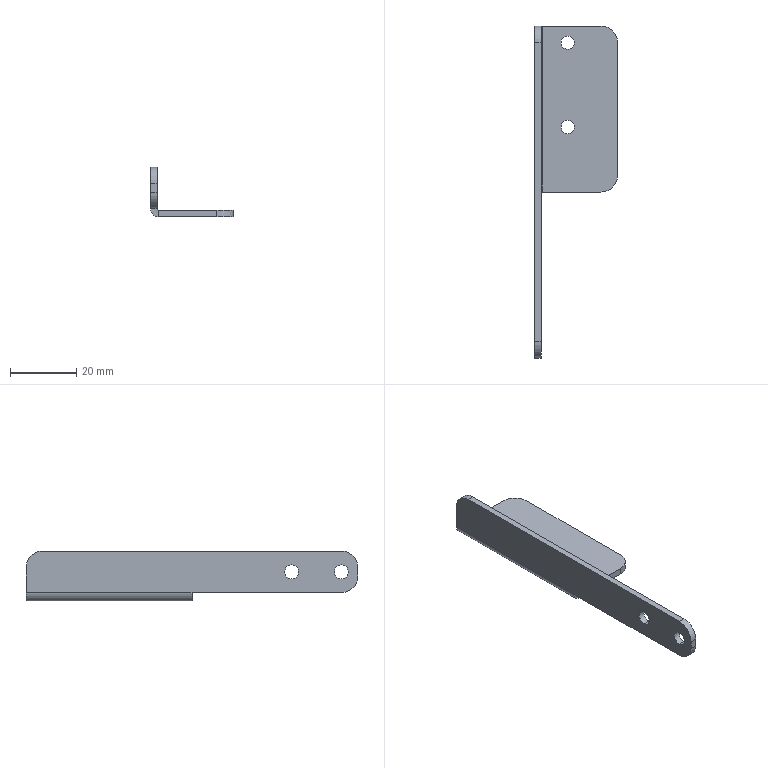Part | SolidWorks | features HoleWzd 2, DeleteBody 1, EdgeFlange 1, Fillet 1, FlatPattern 1, MirrorSolid 1, SMBaseFlange 1, SheetMetal 1 | 1 solid | 28 faces | box 25 x 100 x 15 mm | volume 4826 mm3 | cylinder 15 | plane 13 | commonest cylinder face diameters 10 x5 4 x4 4.2 x4 1 x1 5 x1
STEP:
#1=CARTESIAN_POINT('',(0.,-30.,8.85));
#2=VERTEX_POINT('',#1);
#3=CARTESIAN_POINT('',(0.,-30.,4.65));
#4=VERTEX_POINT('',#3);
#5=CARTESIAN_POINT('',(0.,-30.,6.75));
#6=DIRECTION('',(1.,0.,0.));
#7=DIRECTION('',(0.,0.,-1.));
#8=AXIS2_PLACEMENT_3D('',#5,#6,#7);
#9=CIRCLE('',#8,2.1);
#10=EDGE_CURVE('',#2,#4,#9,.T.);
#11=ORIENTED_EDGE('',*,*,#10,.F.);
#12=CARTESIAN_POINT('',(2.,-30.,8.85));
#13=VERTEX_POINT('',#12);
#14=CARTESIAN_POINT('',(2.,-30.,8.85));
#15=DIRECTION('',(1.,0.,0.));
#16=VECTOR('',#15,1000.);
#17=LINE('',#14,#16);
#18=EDGE_CURVE('',#2,#13,#17,.T.);
#19=ORIENTED_EDGE('',*,*,#18,.T.);
#20=CARTESIAN_POINT('',(2.,-30.,4.65));
#21=VERTEX_POINT('',#20);
#22=CARTESIAN_POINT('',(2.,-30.,6.75));
#23=DIRECTION('',(1.,0.,0.));
#24=DIRECTION('',(0.,0.,-1.));
#25=AXIS2_PLACEMENT_3D('',#22,#23,#24);
#26=CIRCLE('',#25,2.1);
#27=EDGE_CURVE('',#13,#21,#26,.T.);
#28=ORIENTED_EDGE('',*,*,#27,.T.);
#29=CARTESIAN_POINT('',(2.,-30.,4.65));
#30=DIRECTION('',(1.,0.,0.));
#31=VECTOR('',#30,1000.);
#32=LINE('',#29,#31);
#33=EDGE_CURVE('',#4,#21,#32,.T.);
#34=ORIENTED_EDGE('',*,*,#33,.F.);
#35=EDGE_LOOP('',(#11,#19,#28,#34));
#36=FACE_OUTER_BOUND('',#35,.T.);
#37=CARTESIAN_POINT('',(2.,-30.,6.75));
#38=DIRECTION('',(1.,0.,0.));
#39=DIRECTION('',(0.,0.,-1.));
#40=AXIS2_PLACEMENT_3D('',#37,#38,#39);
#41=CYLINDRICAL_SURFACE('',#40,2.1);
#42=ADVANCED_FACE('',(#36),#41,.F.);
#43=CARTESIAN_POINT('',(0.,-45.,8.85));
#44=VERTEX_POINT('',#43);
#45=CARTESIAN_POINT('',(0.,-45.,4.65));
#46=VERTEX_POINT('',#45);
#47=CARTESIAN_POINT('',(0.,-45.,6.75));
#48=DIRECTION('',(1.,0.,0.));
#49=DIRECTION('',(0.,0.,-1.));
#50=AXIS2_PLACEMENT_3D('',#47,#48,#49);
#51=CIRCLE('',#50,2.1);
#52=EDGE_CURVE('',#44,#46,#51,.T.);
#53=ORIENTED_EDGE('',*,*,#52,.F.);
#54=CARTESIAN_POINT('',(2.,-45.,8.85));
#55=VERTEX_POINT('',#54);
#56=CARTESIAN_POINT('',(2.,-45.,8.85));
#57=DIRECTION('',(1.,0.,0.));
#58=VECTOR('',#57,1000.);
#59=LINE('',#56,#58);
#60=EDGE_CURVE('',#44,#55,#59,.T.);
#61=ORIENTED_EDGE('',*,*,#60,.T.);
#62=CARTESIAN_POINT('',(2.,-45.,4.65));
#63=VERTEX_POINT('',#62);
#64=CARTESIAN_POINT('',(2.,-45.,6.75));
#65=DIRECTION('',(1.,0.,0.));
#66=DIRECTION('',(0.,0.,-1.));
#67=AXIS2_PLACEMENT_3D('',#64,#65,#66);
#68=CIRCLE('',#67,2.1);
#69=EDGE_CURVE('',#55,#63,#68,.T.);
#70=ORIENTED_EDGE('',*,*,#69,.T.);
#71=CARTESIAN_POINT('',(2.,-45.,4.65));
#72=DIRECTION('',(1.,0.,0.));
#73=VECTOR('',#72,1000.);
#74=LINE('',#71,#73);
#75=EDGE_CURVE('',#46,#63,#74,.T.);
#76=ORIENTED_EDGE('',*,*,#75,.F.);
#77=EDGE_LOOP('',(#53,#61,#70,#76));
#78=FACE_OUTER_BOUND('',#77,.T.);
#79=CARTESIAN_POINT('',(2.,-45.,6.75));
#80=DIRECTION('',(1.,0.,0.));
#81=DIRECTION('',(0.,0.,-1.));
#82=AXIS2_PLACEMENT_3D('',#79,#80,#81);
#83=CYLINDRICAL_SURFACE('',#82,2.1);
#84=ADVANCED_FACE('',(#78),#83,.F.);
#85=CARTESIAN_POINT('',(8.,45.,-2.));
#86=VERTEX_POINT('',#85);
#87=CARTESIAN_POINT('',(12.,45.,-2.));
#88=VERTEX_POINT('',#87);
#89=CARTESIAN_POINT('',(10.,45.,-2.));
#90=DIRECTION('',(0.,0.,1.));
#91=DIRECTION('',(1.,0.,0.));
#92=AXIS2_PLACEMENT_3D('',#89,#90,#91);
#93=CIRCLE('',#92,2.);
#94=EDGE_CURVE('',#86,#88,#93,.T.);
#95=ORIENTED_EDGE('',*,*,#94,.F.);
#96=CARTESIAN_POINT('',(8.,45.,0.));
#97=VERTEX_POINT('',#96);
#98=CARTESIAN_POINT('',(8.,45.,0.));
#99=DIRECTION('',(0.,0.,1.));
#100=VECTOR('',#99,1000.);
#101=LINE('',#98,#100);
#102=EDGE_CURVE('',#86,#97,#101,.T.);
#103=ORIENTED_EDGE('',*,*,#102,.T.);
#104=CARTESIAN_POINT('',(12.,45.,0.));
#105=VERTEX_POINT('',#104);
#106=CARTESIAN_POINT('',(10.,45.,0.));
#107=DIRECTION('',(0.,0.,1.));
#108=DIRECTION('',(1.,0.,0.));
#109=AXIS2_PLACEMENT_3D('',#106,#107,#108);
#110=CIRCLE('',#109,2.);
#111=EDGE_CURVE('',#97,#105,#110,.T.);
#112=ORIENTED_EDGE('',*,*,#111,.T.);
#113=CARTESIAN_POINT('',(12.,45.,0.));
#114=DIRECTION('',(0.,0.,1.));
#115=VECTOR('',#114,1000.);
#116=LINE('',#113,#115);
#117=EDGE_CURVE('',#88,#105,#116,.T.);
#118=ORIENTED_EDGE('',*,*,#117,.F.);
#119=EDGE_LOOP('',(#95,#103,#112,#118));
#120=FACE_OUTER_BOUND('',#119,.T.);
#121=CARTESIAN_POINT('',(10.,45.,0.));
#122=DIRECTION('',(0.,0.,1.));
#123=DIRECTION('',(1.,0.,0.));
#124=AXIS2_PLACEMENT_3D('',#121,#122,#123);
#125=CYLINDRICAL_SURFACE('',#124,2.);
#126=ADVANCED_FACE('',(#120),#125,.F.);
#127=CARTESIAN_POINT('',(8.,19.6,-2.));
#128=VERTEX_POINT('',#127);
#129=CARTESIAN_POINT('',(12.,19.6,-2.));
#130=VERTEX_POINT('',#129);
#131=CARTESIAN_POINT('',(10.,19.6,-2.));
#132=DIRECTION('',(0.,0.,1.));
#133=DIRECTION('',(1.,0.,0.));
#134=AXIS2_PLACEMENT_3D('',#131,#132,#133);
#135=CIRCLE('',#134,2.);
#136=EDGE_CURVE('',#128,#130,#135,.T.);
#137=ORIENTED_EDGE('',*,*,#136,.F.);
#138=CARTESIAN_POINT('',(8.,19.6,0.));
#139=VERTEX_POINT('',#138);
#140=CARTESIAN_POINT('',(8.,19.6,0.));
#141=DIRECTION('',(0.,0.,1.));
#142=VECTOR('',#141,1000.);
#143=LINE('',#140,#142);
#144=EDGE_CURVE('',#128,#139,#143,.T.);
#145=ORIENTED_EDGE('',*,*,#144,.T.);
#146=CARTESIAN_POINT('',(12.,19.6,0.));
#147=VERTEX_POINT('',#146);
#148=CARTESIAN_POINT('',(10.,19.6,0.));
#149=DIRECTION('',(0.,0.,1.));
#150=DIRECTION('',(1.,0.,0.));
#151=AXIS2_PLACEMENT_3D('',#148,#149,#150);
#152=CIRCLE('',#151,2.);
#153=EDGE_CURVE('',#139,#147,#152,.T.);
#154=ORIENTED_EDGE('',*,*,#153,.T.);
#155=CARTESIAN_POINT('',(12.,19.6,0.));
#156=DIRECTION('',(0.,0.,1.));
#157=VECTOR('',#156,1000.);
#158=LINE('',#155,#157);
#159=EDGE_CURVE('',#130,#147,#158,.T.);
#160=ORIENTED_EDGE('',*,*,#159,.F.);
#161=EDGE_LOOP('',(#137,#145,#154,#160));
#162=FACE_OUTER_BOUND('',#161,.T.);
#163=CARTESIAN_POINT('',(10.,19.6,0.));
#164=DIRECTION('',(0.,0.,1.));
#165=DIRECTION('',(1.,0.,0.));
#166=AXIS2_PLACEMENT_3D('',#163,#164,#165);
#167=CYLINDRICAL_SURFACE('',#166,2.);
#168=ADVANCED_FACE('',(#162),#167,.F.);
#169=CARTESIAN_POINT('',(2.5,0.,-2.));
#170=VERTEX_POINT('',#169);
#171=CARTESIAN_POINT('',(20.,0.,-2.));
#172=VERTEX_POINT('',#171);
#173=CARTESIAN_POINT('',(0.,0.,-2.));
#174=DIRECTION('',(1.,0.,0.));
#175=VECTOR('',#174,1000.);
#176=LINE('',#173,#175);
#177=EDGE_CURVE('',#170,#172,#176,.T.);
#178=ORIENTED_EDGE('',*,*,#177,.T.);
#179=CARTESIAN_POINT('',(20.,0.,0.));
#180=VERTEX_POINT('',#179);
#181=CARTESIAN_POINT('',(20.,0.,-2.));
#182=DIRECTION('',(0.,0.,1.));
#183=VECTOR('',#182,1000.);
#184=LINE('',#181,#183);
#185=EDGE_CURVE('',#172,#180,#184,.T.);
#186=ORIENTED_EDGE('',*,*,#185,.T.);
#187=CARTESIAN_POINT('',(2.5,0.,0.));
#188=VERTEX_POINT('',#187);
#189=CARTESIAN_POINT('',(0.,0.,0.));
#190=DIRECTION('',(1.,0.,0.));
#191=VECTOR('',#190,1000.);
#192=LINE('',#189,#191);
#193=EDGE_CURVE('',#188,#180,#192,.T.);
#194=ORIENTED_EDGE('',*,*,#193,.F.);
#195=CARTESIAN_POINT('',(2.5,0.,0.));
#196=DIRECTION('',(0.,0.,-1.));
#197=VECTOR('',#196,1000.);
#198=LINE('',#195,#197);
#199=EDGE_CURVE('',#188,#170,#198,.T.);
#200=ORIENTED_EDGE('',*,*,#199,.T.);
#201=EDGE_LOOP('',(#178,#186,#194,#200));
#202=FACE_OUTER_BOUND('',#201,.T.);
#203=CARTESIAN_POINT('',(0.,0.,-2.));
#204=DIRECTION('',(0.,-1.,0.));
#205=DIRECTION('',(0.,0.,-1.));
#206=AXIS2_PLACEMENT_3D('',#203,#204,#205);
#207=PLANE('',#206);
#208=ADVANCED_FACE('',(#202),#207,.T.);
#209=CARTESIAN_POINT('',(10.,45.,-2.));
#210=DIRECTION('',(0.,0.,1.));
#211=DIRECTION('',(1.,0.,0.));
#212=AXIS2_PLACEMENT_3D('',#209,#210,#211);
#213=CIRCLE('',#212,2.);
#214=EDGE_CURVE('',#88,#86,#213,.T.);
#215=ORIENTED_EDGE('',*,*,#214,.T.);
#216=ORIENTED_EDGE('',*,*,#94,.T.);
#217=EDGE_LOOP('',(#215,#216));
#218=FACE_BOUND('',#217,.T.);
#219=CARTESIAN_POINT('',(10.,19.6,-2.));
#220=DIRECTION('',(0.,0.,1.));
#221=DIRECTION('',(1.,0.,0.));
#222=AXIS2_PLACEMENT_3D('',#219,#220,#221);
#223=CIRCLE('',#222,2.);
#224=EDGE_CURVE('',#130,#128,#223,.T.);
#225=ORIENTED_EDGE('',*,*,#224,.T.);
#226=ORIENTED_EDGE('',*,*,#136,.T.);
#227=EDGE_LOOP('',(#225,#226));
#228=FACE_BOUND('',#227,.T.);
#229=CARTESIAN_POINT('',(25.,5.,-2.));
#230=VERTEX_POINT('',#229);
#231=CARTESIAN_POINT('',(25.,45.,-2.));
#232=VERTEX_POINT('',#231);
#233=CARTESIAN_POINT('',(25.,50.,-2.));
#234=DIRECTION('',(0.,1.,0.));
#235=VECTOR('',#234,1000.);
#236=LINE('',#233,#235);
#237=EDGE_CURVE('',#230,#232,#236,.T.);
#238=ORIENTED_EDGE('',*,*,#237,.F.);
#239=CARTESIAN_POINT('',(20.,5.,-2.));
#240=DIRECTION('',(0.,0.,-1.));
#241=DIRECTION('',(-1.,0.,0.));
#242=AXIS2_PLACEMENT_3D('',#239,#240,#241);
#243=CIRCLE('',#242,5.);
#244=EDGE_CURVE('',#230,#172,#243,.T.);
#245=ORIENTED_EDGE('',*,*,#244,.T.);
#246=ORIENTED_EDGE('',*,*,#177,.F.);
#247=CARTESIAN_POINT('',(2.5,50.,-2.));
#248=VERTEX_POINT('',#247);
#249=CARTESIAN_POINT('',(2.5,0.,-2.));
#250=DIRECTION('',(0.,1.,0.));
#251=VECTOR('',#250,1000.);
#252=LINE('',#249,#251);
#253=EDGE_CURVE('',#170,#248,#252,.T.);
#254=ORIENTED_EDGE('',*,*,#253,.T.);
#255=CARTESIAN_POINT('',(20.,50.,-2.));
#256=VERTEX_POINT('',#255);
#257=CARTESIAN_POINT('',(0.,50.,-2.));
#258=DIRECTION('',(-1.,0.,0.));
#259=VECTOR('',#258,1000.);
#260=LINE('',#257,#259);
#261=EDGE_CURVE('',#256,#248,#260,.T.);
#262=ORIENTED_EDGE('',*,*,#261,.F.);
#263=CARTESIAN_POINT('',(20.,45.,-2.));
#264=DIRECTION('',(0.,0.,-1.));
#265=DIRECTION('',(-1.,0.,0.));
#266=AXIS2_PLACEMENT_3D('',#263,#264,#265);
#267=CIRCLE('',#266,5.);
#268=EDGE_CURVE('',#256,#232,#267,.T.);
#269=ORIENTED_EDGE('',*,*,#268,.T.);
#270=EDGE_LOOP('',(#238,#245,#246,#254,#262,#269));
#271=FACE_OUTER_BOUND('',#270,.T.);
#272=CARTESIAN_POINT('',(0.,0.,-2.));
#273=DIRECTION('',(0.,0.,-1.));
#274=DIRECTION('',(-1.,0.,0.));
#275=AXIS2_PLACEMENT_3D('',#272,#273,#274);
#276=PLANE('',#275);
#277=ADVANCED_FACE('',(#218,#228,#271),#276,.T.);
#278=CARTESIAN_POINT('',(10.,19.6,0.));
#279=DIRECTION('',(0.,0.,1.));
#280=DIRECTION('',(1.,0.,0.));
#281=AXIS2_PLACEMENT_3D('',#278,#279,#280);
#282=CIRCLE('',#281,2.);
#283=EDGE_CURVE('',#147,#139,#282,.T.);
#284=ORIENTED_EDGE('',*,*,#283,.F.);
#285=ORIENTED_EDGE('',*,*,#153,.F.);
#286=EDGE_LOOP('',(#284,#285));
#287=FACE_BOUND('',#286,.T.);
#288=CARTESIAN_POINT('',(10.,45.,0.));
#289=DIRECTION('',(0.,0.,1.));
#290=DIRECTION('',(1.,0.,0.));
#291=AXIS2_PLACEMENT_3D('',#288,#289,#290);
#292=CIRCLE('',#291,2.);
#293=EDGE_CURVE('',#105,#97,#292,.T.);
#294=ORIENTED_EDGE('',*,*,#293,.F.);
#295=ORIENTED_EDGE('',*,*,#111,.F.);
#296=EDGE_LOOP('',(#294,#295));
#297=FACE_BOUND('',#296,.T.);
#298=ORIENTED_EDGE('',*,*,#193,.T.);
#299=CARTESIAN_POINT('',(25.,5.,0.));
#300=VERTEX_POINT('',#299);
#301=CARTESIAN_POINT('',(20.,5.,0.));
#302=DIRECTION('',(0.,0.,1.));
#303=DIRECTION('',(-1.,0.,0.));
#304=AXIS2_PLACEMENT_3D('',#301,#302,#303);
#305=CIRCLE('',#304,5.);
#306=EDGE_CURVE('',#180,#300,#305,.T.);
#307=ORIENTED_EDGE('',*,*,#306,.T.);
#308=CARTESIAN_POINT('',(25.,45.,0.));
#309=VERTEX_POINT('',#308);
#310=CARTESIAN_POINT('',(25.,50.,0.));
#311=DIRECTION('',(0.,1.,0.));
#312=VECTOR('',#311,1000.);
#313=LINE('',#310,#312);
#314=EDGE_CURVE('',#300,#309,#313,.T.);
#315=ORIENTED_EDGE('',*,*,#314,.T.);
#316=CARTESIAN_POINT('',(20.,50.,0.));
#317=VERTEX_POINT('',#316);
#318=CARTESIAN_POINT('',(20.,45.,0.));
#319=DIRECTION('',(0.,0.,1.));
#320=DIRECTION('',(-1.,0.,0.));
#321=AXIS2_PLACEMENT_3D('',#318,#319,#320);
#322=CIRCLE('',#321,5.);
#323=EDGE_CURVE('',#309,#317,#322,.T.);
#324=ORIENTED_EDGE('',*,*,#323,.T.);
#325=CARTESIAN_POINT('',(2.5,50.,0.));
#326=VERTEX_POINT('',#325);
#327=CARTESIAN_POINT('',(0.,50.,0.));
#328=DIRECTION('',(-1.,0.,0.));
#329=VECTOR('',#328,1000.);
#330=LINE('',#327,#329);
#331=EDGE_CURVE('',#317,#326,#330,.T.);
#332=ORIENTED_EDGE('',*,*,#331,.T.);
#333=CARTESIAN_POINT('',(2.5,0.,0.));
#334=DIRECTION('',(0.,1.,0.));
#335=VECTOR('',#334,1000.);
#336=LINE('',#333,#335);
#337=EDGE_CURVE('',#188,#326,#336,.T.);
#338=ORIENTED_EDGE('',*,*,#337,.F.);
#339=EDGE_LOOP('',(#298,#307,#315,#324,#332,#338));
#340=FACE_OUTER_BOUND('',#339,.T.);
#341=CARTESIAN_POINT('',(0.,0.,0.));
#342=DIRECTION('',(0.,0.,-1.));
#343=DIRECTION('',(-1.,0.,0.));
#344=AXIS2_PLACEMENT_3D('',#341,#342,#343);
#345=PLANE('',#344);
#346=ADVANCED_FACE('',(#287,#297,#340),#345,.F.);
#347=ORIENTED_EDGE('',*,*,#331,.F.);
#348=CARTESIAN_POINT('',(20.,50.,-2.));
#349=DIRECTION('',(0.,0.,-1.));
#350=VECTOR('',#349,1000.);
#351=LINE('',#348,#350);
#352=EDGE_CURVE('',#317,#256,#351,.T.);
#353=ORIENTED_EDGE('',*,*,#352,.T.);
#354=ORIENTED_EDGE('',*,*,#261,.T.);
#355=CARTESIAN_POINT('',(2.5,50.,0.));
#356=DIRECTION('',(0.,0.,-1.));
#357=VECTOR('',#356,1000.);
#358=LINE('',#355,#357);
#359=EDGE_CURVE('',#326,#248,#358,.T.);
#360=ORIENTED_EDGE('',*,*,#359,.F.);
#361=EDGE_LOOP('',(#347,#353,#354,#360));
#362=FACE_OUTER_BOUND('',#361,.T.);
#363=CARTESIAN_POINT('',(0.,50.,-2.));
#364=DIRECTION('',(0.,1.,0.));
#365=DIRECTION('',(0.,0.,1.));
#366=AXIS2_PLACEMENT_3D('',#363,#364,#365);
#367=PLANE('',#366);
#368=ADVANCED_FACE('',(#362),#367,.T.);
#369=ORIENTED_EDGE('',*,*,#314,.F.);
#370=CARTESIAN_POINT('',(25.,5.,-2.));
#371=DIRECTION('',(0.,0.,-1.));
#372=VECTOR('',#371,1000.);
#373=LINE('',#370,#372);
#374=EDGE_CURVE('',#300,#230,#373,.T.);
#375=ORIENTED_EDGE('',*,*,#374,.T.);
#376=ORIENTED_EDGE('',*,*,#237,.T.);
#377=CARTESIAN_POINT('',(25.,45.,-2.));
#378=DIRECTION('',(0.,0.,1.));
#379=VECTOR('',#378,1000.);
#380=LINE('',#377,#379);
#381=EDGE_CURVE('',#232,#309,#380,.T.);
#382=ORIENTED_EDGE('',*,*,#381,.T.);
#383=EDGE_LOOP('',(#369,#375,#376,#382));
#384=FACE_OUTER_BOUND('',#383,.T.);
#385=CARTESIAN_POINT('',(25.,50.,-2.));
#386=DIRECTION('',(1.,0.,0.));
#387=DIRECTION('',(0.,1.,0.));
#388=AXIS2_PLACEMENT_3D('',#385,#386,#387);
#389=PLANE('',#388);
#390=ADVANCED_FACE('',(#384),#389,.T.);
#391=ORIENTED_EDGE('',*,*,#144,.F.);
#392=ORIENTED_EDGE('',*,*,#224,.F.);
#393=ORIENTED_EDGE('',*,*,#159,.T.);
#394=ORIENTED_EDGE('',*,*,#283,.T.);
#395=EDGE_LOOP('',(#391,#392,#393,#394));
#396=FACE_OUTER_BOUND('',#395,.T.);
#397=CARTESIAN_POINT('',(10.,19.6,0.));
#398=DIRECTION('',(0.,0.,1.));
#399=DIRECTION('',(1.,0.,0.));
#400=AXIS2_PLACEMENT_3D('',#397,#398,#399);
#401=CYLINDRICAL_SURFACE('',#400,2.);
#402=ADVANCED_FACE('',(#396),#401,.F.);
#403=ORIENTED_EDGE('',*,*,#102,.F.);
#404=ORIENTED_EDGE('',*,*,#214,.F.);
#405=ORIENTED_EDGE('',*,*,#117,.T.);
#406=ORIENTED_EDGE('',*,*,#293,.T.);
#407=EDGE_LOOP('',(#403,#404,#405,#406));
#408=FACE_OUTER_BOUND('',#407,.T.);
#409=CARTESIAN_POINT('',(10.,45.,0.));
#410=DIRECTION('',(0.,0.,1.));
#411=DIRECTION('',(1.,0.,0.));
#412=AXIS2_PLACEMENT_3D('',#409,#410,#411);
#413=CYLINDRICAL_SURFACE('',#412,2.);
#414=ADVANCED_FACE('',(#408),#413,.F.);
#415=CARTESIAN_POINT('',(2.,50.,0.5));
#416=VERTEX_POINT('',#415);
#417=CARTESIAN_POINT('',(0.,50.,0.5));
#418=VERTEX_POINT('',#417);
#419=CARTESIAN_POINT('',(0.,50.,0.5));
#420=DIRECTION('',(-1.,0.,0.));
#421=VECTOR('',#420,1000.);
#422=LINE('',#419,#421);
#423=EDGE_CURVE('',#416,#418,#422,.T.);
#424=ORIENTED_EDGE('',*,*,#423,.F.);
#425=CARTESIAN_POINT('',(2.5,50.,0.5));
#426=DIRECTION('',(0.,1.,0.));
#427=DIRECTION('',(0.,0.,-1.));
#428=AXIS2_PLACEMENT_3D('',#425,#426,#427);
#429=CIRCLE('',#428,0.5);
#430=EDGE_CURVE('',#326,#416,#429,.T.);
#431=ORIENTED_EDGE('',*,*,#430,.F.);
#432=ORIENTED_EDGE('',*,*,#359,.T.);
#433=CARTESIAN_POINT('',(2.5,50.,0.5));
#434=DIRECTION('',(0.,1.,0.));
#435=DIRECTION('',(0.,0.,-1.));
#436=AXIS2_PLACEMENT_3D('',#433,#434,#435);
#437=CIRCLE('',#436,2.5);
#438=EDGE_CURVE('',#248,#418,#437,.T.);
#439=ORIENTED_EDGE('',*,*,#438,.T.);
#440=EDGE_LOOP('',(#424,#431,#432,#439));
#441=FACE_OUTER_BOUND('',#440,.T.);
#442=CARTESIAN_POINT('',(2.5,50.,0.5));
#443=DIRECTION('',(0.,1.,0.));
#444=DIRECTION('',(0.,0.,1.));
#445=AXIS2_PLACEMENT_3D('',#442,#443,#444);
#446=PLANE('',#445);
#447=ADVANCED_FACE('',(#441),#446,.T.);
#448=CARTESIAN_POINT('',(2.,0.,0.5));
#449=VERTEX_POINT('',#448);
#450=CARTESIAN_POINT('',(2.5,0.,0.5));
#451=DIRECTION('',(0.,-1.,0.));
#452=DIRECTION('',(0.,0.,-1.));
#453=AXIS2_PLACEMENT_3D('',#450,#451,#452);
#454=CIRCLE('',#453,0.5);
#455=EDGE_CURVE('',#449,#188,#454,.T.);
#456=ORIENTED_EDGE('',*,*,#455,.F.);
#457=CARTESIAN_POINT('',(0.,0.,0.5));
#458=VERTEX_POINT('',#457);
#459=CARTESIAN_POINT('',(2.,0.,0.5));
#460=DIRECTION('',(-1.,0.,0.));
#461=VECTOR('',#460,1000.);
#462=LINE('',#459,#461);
#463=EDGE_CURVE('',#449,#458,#462,.T.);
#464=ORIENTED_EDGE('',*,*,#463,.T.);
#465=CARTESIAN_POINT('',(2.5,0.,0.5));
#466=DIRECTION('',(0.,-1.,0.));
#467=DIRECTION('',(0.,0.,-1.));
#468=AXIS2_PLACEMENT_3D('',#465,#466,#467);
#469=CIRCLE('',#468,2.5);
#470=EDGE_CURVE('',#458,#170,#469,.T.);
#471=ORIENTED_EDGE('',*,*,#470,.T.);
#472=ORIENTED_EDGE('',*,*,#199,.F.);
#473=EDGE_LOOP('',(#456,#464,#471,#472));
#474=FACE_OUTER_BOUND('',#473,.T.);
#475=CARTESIAN_POINT('',(2.5,0.,0.5));
#476=DIRECTION('',(0.,1.,0.));
#477=DIRECTION('',(0.,0.,1.));
#478=AXIS2_PLACEMENT_3D('',#475,#476,#477);
#479=PLANE('',#478);
#480=ADVANCED_FACE('',(#474),#479,.F.);
#481=ORIENTED_EDGE('',*,*,#253,.F.);
#482=ORIENTED_EDGE('',*,*,#470,.F.);
#483=CARTESIAN_POINT('',(0.,0.,0.5));
#484=DIRECTION('',(0.,-1.,0.));
#485=VECTOR('',#484,1000.);
#486=LINE('',#483,#485);
#487=EDGE_CURVE('',#418,#458,#486,.T.);
#488=ORIENTED_EDGE('',*,*,#487,.F.);
#489=ORIENTED_EDGE('',*,*,#438,.F.);
#490=EDGE_LOOP('',(#481,#482,#488,#489));
#491=FACE_OUTER_BOUND('',#490,.T.);
#492=CARTESIAN_POINT('',(2.5,0.,0.5));
#493=DIRECTION('',(0.,-1.,0.));
#494=DIRECTION('',(-1.,0.,0.));
#495=AXIS2_PLACEMENT_3D('',#492,#493,#494);
#496=CYLINDRICAL_SURFACE('',#495,2.5);
#497=ADVANCED_FACE('',(#491),#496,.T.);
#498=ORIENTED_EDGE('',*,*,#337,.T.);
#499=ORIENTED_EDGE('',*,*,#430,.T.);
#500=CARTESIAN_POINT('',(2.,50.,0.5));
#501=DIRECTION('',(0.,-1.,0.));
#502=VECTOR('',#501,1000.);
#503=LINE('',#500,#502);
#504=EDGE_CURVE('',#416,#449,#503,.T.);
#505=ORIENTED_EDGE('',*,*,#504,.T.);
#506=ORIENTED_EDGE('',*,*,#455,.T.);
#507=EDGE_LOOP('',(#498,#499,#505,#506));
#508=FACE_OUTER_BOUND('',#507,.T.);
#509=CARTESIAN_POINT('',(2.5,0.,0.5));
#510=DIRECTION('',(0.,-1.,0.));
#511=DIRECTION('',(-1.,0.,0.));
#512=AXIS2_PLACEMENT_3D('',#509,#510,#511);
#513=CYLINDRICAL_SURFACE('',#512,0.5);
#514=ADVANCED_FACE('',(#508),#513,.F.);
#515=CARTESIAN_POINT('',(2.,-45.,0.5));
#516=VERTEX_POINT('',#515);
#517=CARTESIAN_POINT('',(2.,50.,0.5));
#518=DIRECTION('',(0.,-1.,0.));
#519=VECTOR('',#518,1000.);
#520=LINE('',#517,#519);
#521=EDGE_CURVE('',#449,#516,#520,.T.);
#522=ORIENTED_EDGE('',*,*,#521,.T.);
#523=CARTESIAN_POINT('',(0.,-45.,0.5));
#524=VERTEX_POINT('',#523);
#525=CARTESIAN_POINT('',(0.,-45.,0.5));
#526=DIRECTION('',(-1.,0.,0.));
#527=VECTOR('',#526,1000.);
#528=LINE('',#525,#527);
#529=EDGE_CURVE('',#516,#524,#528,.T.);
#530=ORIENTED_EDGE('',*,*,#529,.T.);
#531=CARTESIAN_POINT('',(0.,50.,0.5));
#532=DIRECTION('',(0.,1.,0.));
#533=VECTOR('',#532,1000.);
#534=LINE('',#531,#533);
#535=EDGE_CURVE('',#524,#458,#534,.T.);
#536=ORIENTED_EDGE('',*,*,#535,.T.);
#537=ORIENTED_EDGE('',*,*,#463,.F.);
#538=EDGE_LOOP('',(#522,#530,#536,#537));
#539=FACE_OUTER_BOUND('',#538,.T.);
#540=CARTESIAN_POINT('',(2.,50.,0.5));
#541=DIRECTION('',(0.,0.,-1.));
#542=DIRECTION('',(-1.,0.,0.));
#543=AXIS2_PLACEMENT_3D('',#540,#541,#542);
#544=PLANE('',#543);
#545=ADVANCED_FACE('',(#539),#544,.T.);
#546=CARTESIAN_POINT('',(0.,50.,8.));
#547=VERTEX_POINT('',#546);
#548=CARTESIAN_POINT('',(0.,50.,0.));
#549=DIRECTION('',(0.,0.,-1.));
#550=VECTOR('',#549,1000.);
#551=LINE('',#548,#550);
#552=EDGE_CURVE('',#547,#418,#551,.T.);
#553=ORIENTED_EDGE('',*,*,#552,.F.);
#554=CARTESIAN_POINT('',(2.,50.,8.));
#555=VERTEX_POINT('',#554);
#556=CARTESIAN_POINT('',(0.,50.,8.));
#557=DIRECTION('',(1.,0.,0.));
#558=VECTOR('',#557,1000.);
#559=LINE('',#556,#558);
#560=EDGE_CURVE('',#547,#555,#559,.T.);
#561=ORIENTED_EDGE('',*,*,#560,.T.);
#562=CARTESIAN_POINT('',(2.,50.,0.));
#563=DIRECTION('',(0.,0.,-1.));
#564=VECTOR('',#563,1000.);
#565=LINE('',#562,#564);
#566=EDGE_CURVE('',#555,#416,#565,.T.);
#567=ORIENTED_EDGE('',*,*,#566,.T.);
#568=ORIENTED_EDGE('',*,*,#423,.T.);
#569=EDGE_LOOP('',(#553,#561,#567,#568));
#570=FACE_OUTER_BOUND('',#569,.T.);
#571=CARTESIAN_POINT('',(0.,50.,0.));
#572=DIRECTION('',(0.,-1.,0.));
#573=DIRECTION('',(0.,0.,-1.));
#574=AXIS2_PLACEMENT_3D('',#571,#572,#573);
#575=PLANE('',#574);
#576=ADVANCED_FACE('',(#570),#575,.F.);
#577=CARTESIAN_POINT('',(0.,-50.,5.5));
#578=VERTEX_POINT('',#577);
#579=CARTESIAN_POINT('',(0.,-50.,8.));
#580=VERTEX_POINT('',#579);
#581=CARTESIAN_POINT('',(0.,-50.,0.));
#582=DIRECTION('',(0.,0.,1.));
#583=VECTOR('',#582,1000.);
#584=LINE('',#581,#583);
#585=EDGE_CURVE('',#578,#580,#584,.T.);
#586=ORIENTED_EDGE('',*,*,#585,.F.);
#587=CARTESIAN_POINT('',(2.,-50.,5.5));
#588=VERTEX_POINT('',#587);
#589=CARTESIAN_POINT('',(2.,-50.,5.5));
#590=DIRECTION('',(1.,0.,0.));
#591=VECTOR('',#590,1000.);
#592=LINE('',#589,#591);
#593=EDGE_CURVE('',#578,#588,#592,.T.);
#594=ORIENTED_EDGE('',*,*,#593,.T.);
#595=CARTESIAN_POINT('',(2.,-50.,8.));
#596=VERTEX_POINT('',#595);
#597=CARTESIAN_POINT('',(2.,-50.,13.));
#598=DIRECTION('',(0.,0.,1.));
#599=VECTOR('',#598,1000.);
#600=LINE('',#597,#599);
#601=EDGE_CURVE('',#588,#596,#600,.T.);
#602=ORIENTED_EDGE('',*,*,#601,.T.);
#603=CARTESIAN_POINT('',(0.,-50.,8.));
#604=DIRECTION('',(-1.,0.,0.));
#605=VECTOR('',#604,1000.);
#606=LINE('',#603,#605);
#607=EDGE_CURVE('',#596,#580,#606,.T.);
#608=ORIENTED_EDGE('',*,*,#607,.T.);
#609=EDGE_LOOP('',(#586,#594,#602,#608));
#610=FACE_OUTER_BOUND('',#609,.T.);
#611=CARTESIAN_POINT('',(0.,-50.,13.));
#612=DIRECTION('',(0.,1.,0.));
#613=DIRECTION('',(0.,0.,1.));
#614=AXIS2_PLACEMENT_3D('',#611,#612,#613);
#615=PLANE('',#614);
#616=ADVANCED_FACE('',(#610),#615,.F.);
#617=CARTESIAN_POINT('',(0.,-30.,6.75));
#618=DIRECTION('',(1.,0.,0.));
#619=DIRECTION('',(0.,0.,-1.));
#620=AXIS2_PLACEMENT_3D('',#617,#618,#619);
#621=CIRCLE('',#620,2.1);
#622=EDGE_CURVE('',#4,#2,#621,.T.);
#623=ORIENTED_EDGE('',*,*,#622,.T.);
#624=ORIENTED_EDGE('',*,*,#10,.T.);
#625=EDGE_LOOP('',(#623,#624));
#626=FACE_BOUND('',#625,.T.);
#627=CARTESIAN_POINT('',(0.,-45.,6.75));
#628=DIRECTION('',(1.,0.,0.));
#629=DIRECTION('',(0.,0.,-1.));
#630=AXIS2_PLACEMENT_3D('',#627,#628,#629);
#631=CIRCLE('',#630,2.1);
#632=EDGE_CURVE('',#46,#44,#631,.T.);
#633=ORIENTED_EDGE('',*,*,#632,.T.);
#634=ORIENTED_EDGE('',*,*,#52,.T.);
#635=EDGE_LOOP('',(#633,#634));
#636=FACE_BOUND('',#635,.T.);
#637=ORIENTED_EDGE('',*,*,#535,.F.);
#638=CARTESIAN_POINT('',(0.,-45.,5.5));
#639=DIRECTION('',(-1.,0.,0.));
#640=DIRECTION('',(0.,0.,-1.));
#641=AXIS2_PLACEMENT_3D('',#638,#639,#640);
#642=CIRCLE('',#641,5.);
#643=EDGE_CURVE('',#524,#578,#642,.T.);
#644=ORIENTED_EDGE('',*,*,#643,.T.);
#645=ORIENTED_EDGE('',*,*,#585,.T.);
#646=CARTESIAN_POINT('',(0.,-45.,13.));
#647=VERTEX_POINT('',#646);
#648=CARTESIAN_POINT('',(0.,-45.,8.));
#649=DIRECTION('',(-1.,0.,0.));
#650=DIRECTION('',(0.,0.,-1.));
#651=AXIS2_PLACEMENT_3D('',#648,#649,#650);
#652=CIRCLE('',#651,5.);
#653=EDGE_CURVE('',#580,#647,#652,.T.);
#654=ORIENTED_EDGE('',*,*,#653,.T.);
#655=CARTESIAN_POINT('',(0.,45.,13.));
#656=VERTEX_POINT('',#655);
#657=CARTESIAN_POINT('',(0.,0.,13.));
#658=DIRECTION('',(0.,1.,0.));
#659=VECTOR('',#658,1000.);
#660=LINE('',#657,#659);
#661=EDGE_CURVE('',#647,#656,#660,.T.);
#662=ORIENTED_EDGE('',*,*,#661,.T.);
#663=CARTESIAN_POINT('',(0.,45.,8.));
#664=DIRECTION('',(-1.,0.,0.));
#665=DIRECTION('',(0.,0.,-1.));
#666=AXIS2_PLACEMENT_3D('',#663,#664,#665);
#667=CIRCLE('',#666,5.);
#668=EDGE_CURVE('',#656,#547,#667,.T.);
#669=ORIENTED_EDGE('',*,*,#668,.T.);
#670=ORIENTED_EDGE('',*,*,#552,.T.);
#671=ORIENTED_EDGE('',*,*,#487,.T.);
#672=EDGE_LOOP('',(#637,#644,#645,#654,#662,#669,#670,#671));
#673=FACE_OUTER_BOUND('',#672,.T.);
#674=CARTESIAN_POINT('',(0.,0.,0.));
#675=DIRECTION('',(1.,0.,0.));
#676=DIRECTION('',(0.,0.,-1.));
#677=AXIS2_PLACEMENT_3D('',#674,#675,#676);
#678=PLANE('',#677);
#679=ADVANCED_FACE('',(#626,#636,#673),#678,.F.);
#680=CARTESIAN_POINT('',(2.,-30.,6.75));
#681=DIRECTION('',(1.,0.,0.));
#682=DIRECTION('',(0.,0.,-1.));
#683=AXIS2_PLACEMENT_3D('',#680,#681,#682);
#684=CIRCLE('',#683,2.1);
#685=EDGE_CURVE('',#21,#13,#684,.T.);
#686=ORIENTED_EDGE('',*,*,#685,.F.);
#687=ORIENTED_EDGE('',*,*,#27,.F.);
#688=EDGE_LOOP('',(#686,#687));
#689=FACE_BOUND('',#688,.T.);
#690=CARTESIAN_POINT('',(2.,-45.,6.75));
#691=DIRECTION('',(1.,0.,0.));
#692=DIRECTION('',(0.,0.,-1.));
#693=AXIS2_PLACEMENT_3D('',#690,#691,#692);
#694=CIRCLE('',#693,2.1);
#695=EDGE_CURVE('',#63,#55,#694,.T.);
#696=ORIENTED_EDGE('',*,*,#695,.F.);
#697=ORIENTED_EDGE('',*,*,#69,.F.);
#698=EDGE_LOOP('',(#696,#697));
#699=FACE_BOUND('',#698,.T.);
#700=ORIENTED_EDGE('',*,*,#601,.F.);
#701=CARTESIAN_POINT('',(2.,-45.,5.5));
#702=DIRECTION('',(1.,0.,0.));
#703=DIRECTION('',(0.,0.,-1.));
#704=AXIS2_PLACEMENT_3D('',#701,#702,#703);
#705=CIRCLE('',#704,5.);
#706=EDGE_CURVE('',#588,#516,#705,.T.);
#707=ORIENTED_EDGE('',*,*,#706,.T.);
#708=ORIENTED_EDGE('',*,*,#521,.F.);
#709=ORIENTED_EDGE('',*,*,#504,.F.);
#710=ORIENTED_EDGE('',*,*,#566,.F.);
#711=CARTESIAN_POINT('',(2.,45.,13.));
#712=VERTEX_POINT('',#711);
#713=CARTESIAN_POINT('',(2.,45.,8.));
#714=DIRECTION('',(1.,0.,0.));
#715=DIRECTION('',(0.,0.,-1.));
#716=AXIS2_PLACEMENT_3D('',#713,#714,#715);
#717=CIRCLE('',#716,5.);
#718=EDGE_CURVE('',#555,#712,#717,.T.);
#719=ORIENTED_EDGE('',*,*,#718,.T.);
#720=CARTESIAN_POINT('',(2.,-45.,13.));
#721=VERTEX_POINT('',#720);
#722=CARTESIAN_POINT('',(2.,50.,13.));
#723=DIRECTION('',(0.,1.,0.));
#724=VECTOR('',#723,1000.);
#725=LINE('',#722,#724);
#726=EDGE_CURVE('',#721,#712,#725,.T.);
#727=ORIENTED_EDGE('',*,*,#726,.F.);
#728=CARTESIAN_POINT('',(2.,-45.,8.));
#729=DIRECTION('',(1.,0.,0.));
#730=DIRECTION('',(0.,0.,-1.));
#731=AXIS2_PLACEMENT_3D('',#728,#729,#730);
#732=CIRCLE('',#731,5.);
#733=EDGE_CURVE('',#721,#596,#732,.T.);
#734=ORIENTED_EDGE('',*,*,#733,.T.);
#735=EDGE_LOOP('',(#700,#707,#708,#709,#710,#719,#727,#734));
#736=FACE_OUTER_BOUND('',#735,.T.);
#737=CARTESIAN_POINT('',(2.,0.,0.));
#738=DIRECTION('',(1.,0.,0.));
#739=DIRECTION('',(0.,0.,-1.));
#740=AXIS2_PLACEMENT_3D('',#737,#738,#739);
#741=PLANE('',#740);
#742=ADVANCED_FACE('',(#689,#699,#736),#741,.T.);
#743=ORIENTED_EDGE('',*,*,#661,.F.);
#744=CARTESIAN_POINT('',(0.,-45.,13.));
#745=DIRECTION('',(1.,0.,0.));
#746=VECTOR('',#745,1000.);
#747=LINE('',#744,#746);
#748=EDGE_CURVE('',#647,#721,#747,.T.);
#749=ORIENTED_EDGE('',*,*,#748,.T.);
#750=ORIENTED_EDGE('',*,*,#726,.T.);
#751=CARTESIAN_POINT('',(0.,45.,13.));
#752=DIRECTION('',(-1.,0.,0.));
#753=VECTOR('',#752,1000.);
#754=LINE('',#751,#753);
#755=EDGE_CURVE('',#712,#656,#754,.T.);
#756=ORIENTED_EDGE('',*,*,#755,.T.);
#757=EDGE_LOOP('',(#743,#749,#750,#756));
#758=FACE_OUTER_BOUND('',#757,.T.);
#759=CARTESIAN_POINT('',(0.,50.,13.));
#760=DIRECTION('',(0.,0.,-1.));
#761=DIRECTION('',(-1.,0.,0.));
#762=AXIS2_PLACEMENT_3D('',#759,#760,#761);
#763=PLANE('',#762);
#764=ADVANCED_FACE('',(#758),#763,.F.);
#765=ORIENTED_EDGE('',*,*,#60,.F.);
#766=ORIENTED_EDGE('',*,*,#632,.F.);
#767=ORIENTED_EDGE('',*,*,#75,.T.);
#768=ORIENTED_EDGE('',*,*,#695,.T.);
#769=EDGE_LOOP('',(#765,#766,#767,#768));
#770=FACE_OUTER_BOUND('',#769,.T.);
#771=CARTESIAN_POINT('',(2.,-45.,6.75));
#772=DIRECTION('',(1.,0.,0.));
#773=DIRECTION('',(0.,0.,-1.));
#774=AXIS2_PLACEMENT_3D('',#771,#772,#773);
#775=CYLINDRICAL_SURFACE('',#774,2.1);
#776=ADVANCED_FACE('',(#770),#775,.F.);
#777=ORIENTED_EDGE('',*,*,#18,.F.);
#778=ORIENTED_EDGE('',*,*,#622,.F.);
#779=ORIENTED_EDGE('',*,*,#33,.T.);
#780=ORIENTED_EDGE('',*,*,#685,.T.);
#781=EDGE_LOOP('',(#777,#778,#779,#780));
#782=FACE_OUTER_BOUND('',#781,.T.);
#783=CARTESIAN_POINT('',(2.,-30.,6.75));
#784=DIRECTION('',(1.,0.,0.));
#785=DIRECTION('',(0.,0.,-1.));
#786=AXIS2_PLACEMENT_3D('',#783,#784,#785);
#787=CYLINDRICAL_SURFACE('',#786,2.1);
#788=ADVANCED_FACE('',(#782),#787,.F.);
#789=ORIENTED_EDGE('',*,*,#244,.F.);
#790=ORIENTED_EDGE('',*,*,#374,.F.);
#791=ORIENTED_EDGE('',*,*,#306,.F.);
#792=ORIENTED_EDGE('',*,*,#185,.F.);
#793=EDGE_LOOP('',(#789,#790,#791,#792));
#794=FACE_OUTER_BOUND('',#793,.T.);
#795=CARTESIAN_POINT('',(20.,5.,-2.));
#796=DIRECTION('',(0.,0.,1.));
#797=DIRECTION('',(1.,0.,0.));
#798=AXIS2_PLACEMENT_3D('',#795,#796,#797);
#799=CYLINDRICAL_SURFACE('',#798,5.);
#800=ADVANCED_FACE('',(#794),#799,.T.);
#801=ORIENTED_EDGE('',*,*,#268,.F.);
#802=ORIENTED_EDGE('',*,*,#352,.F.);
#803=ORIENTED_EDGE('',*,*,#323,.F.);
#804=ORIENTED_EDGE('',*,*,#381,.F.);
#805=EDGE_LOOP('',(#801,#802,#803,#804));
#806=FACE_OUTER_BOUND('',#805,.T.);
#807=CARTESIAN_POINT('',(20.,45.,-2.));
#808=DIRECTION('',(0.,0.,1.));
#809=DIRECTION('',(1.,0.,0.));
#810=AXIS2_PLACEMENT_3D('',#807,#808,#809);
#811=CYLINDRICAL_SURFACE('',#810,5.);
#812=ADVANCED_FACE('',(#806),#811,.T.);
#813=ORIENTED_EDGE('',*,*,#706,.F.);
#814=ORIENTED_EDGE('',*,*,#593,.F.);
#815=ORIENTED_EDGE('',*,*,#643,.F.);
#816=ORIENTED_EDGE('',*,*,#529,.F.);
#817=EDGE_LOOP('',(#813,#814,#815,#816));
#818=FACE_OUTER_BOUND('',#817,.T.);
#819=CARTESIAN_POINT('',(2.,-45.,5.5));
#820=DIRECTION('',(1.,0.,0.));
#821=DIRECTION('',(0.,0.,-1.));
#822=AXIS2_PLACEMENT_3D('',#819,#820,#821);
#823=CYLINDRICAL_SURFACE('',#822,5.);
#824=ADVANCED_FACE('',(#818),#823,.T.);
#825=ORIENTED_EDGE('',*,*,#653,.F.);
#826=ORIENTED_EDGE('',*,*,#607,.F.);
#827=ORIENTED_EDGE('',*,*,#733,.F.);
#828=ORIENTED_EDGE('',*,*,#748,.F.);
#829=EDGE_LOOP('',(#825,#826,#827,#828));
#830=FACE_OUTER_BOUND('',#829,.T.);
#831=CARTESIAN_POINT('',(0.,-45.,8.));
#832=DIRECTION('',(1.,0.,0.));
#833=DIRECTION('',(0.,0.,-1.));
#834=AXIS2_PLACEMENT_3D('',#831,#832,#833);
#835=CYLINDRICAL_SURFACE('',#834,5.);
#836=ADVANCED_FACE('',(#830),#835,.T.);
#837=ORIENTED_EDGE('',*,*,#668,.F.);
#838=ORIENTED_EDGE('',*,*,#755,.F.);
#839=ORIENTED_EDGE('',*,*,#718,.F.);
#840=ORIENTED_EDGE('',*,*,#560,.F.);
#841=EDGE_LOOP('',(#837,#838,#839,#840));
#842=FACE_OUTER_BOUND('',#841,.T.);
#843=CARTESIAN_POINT('',(0.,45.,8.));
#844=DIRECTION('',(1.,0.,0.));
#845=DIRECTION('',(0.,0.,-1.));
#846=AXIS2_PLACEMENT_3D('',#843,#844,#845);
#847=CYLINDRICAL_SURFACE('',#846,5.);
#848=ADVANCED_FACE('',(#842),#847,.T.);
#849=CLOSED_SHELL('',(#42,#84,#126,#168,#208,#277,#346,#368,#390,#402,#414,#447,#480,#497,#514,#545,#576,#616,#679,#742,#764,#776,#788,#800,#812,#824,#836,#848));
#850=MANIFOLD_SOLID_BREP('',#849);
#851=CARTESIAN_POINT('',(0.,0.,0.));
#852=DIRECTION('',(0.,0.,1.));
#853=DIRECTION('',(1.,0.,0.));
#854=AXIS2_PLACEMENT_3D('',#851,#852,#853);
#855=(LENGTH_UNIT()NAMED_UNIT(*)SI_UNIT(.MILLI.,.METRE.));
#856=UNCERTAINTY_MEASURE_WITH_UNIT(LENGTH_MEASURE(0.00001),#855,'','');
#857=(NAMED_UNIT(*)PLANE_ANGLE_UNIT()SI_UNIT($,.RADIAN.));
#858=(NAMED_UNIT(*)SI_UNIT($,.STERADIAN.)SOLID_ANGLE_UNIT());
#859=(GEOMETRIC_REPRESENTATION_CONTEXT(3)GLOBAL_UNCERTAINTY_ASSIGNED_CONTEXT((#856))GLOBAL_UNIT_ASSIGNED_CONTEXT((#855,#857,#858))REPRESENTATION_CONTEXT('',''));
#860=ADVANCED_BREP_SHAPE_REPRESENTATION('',(#850,#854),#859);